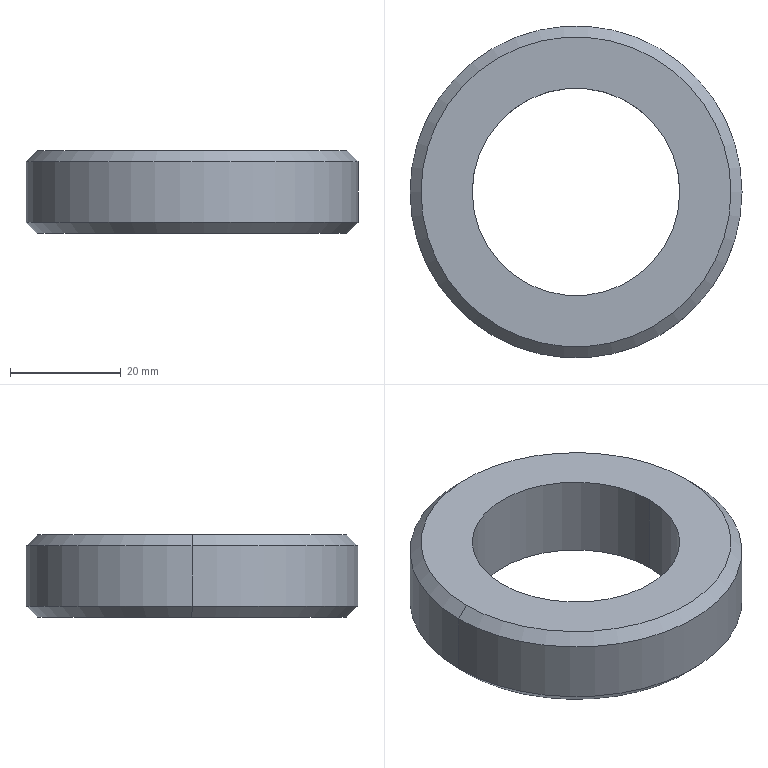Part | SolidWorks | features Chamfer 1, Extrusion 1, HoleWzd 1, ICE 1 | 1 solid | 10 faces | box 60 x 60 x 15 mm | volume 25107 mm3 | cylinder 4 | cone 4 | plane 2 | commonest cylinder face diameters 37.5 x2 60 x2
STEP:
#1=CARTESIAN_POINT('',(-18.75,0.,0.));
#2=VERTEX_POINT('',#1);
#3=CARTESIAN_POINT('',(18.75,0.,0.));
#4=VERTEX_POINT('',#3);
#5=CARTESIAN_POINT('',(0.,0.,0.));
#6=DIRECTION('',(0.,0.,1.));
#7=DIRECTION('',(1.,0.,0.));
#8=AXIS2_PLACEMENT_3D('',#5,#6,#7);
#9=CIRCLE('',#8,18.75);
#10=EDGE_CURVE('',#2,#4,#9,.T.);
#11=ORIENTED_EDGE('',*,*,#10,.F.);
#12=CARTESIAN_POINT('',(-18.75,0.,15.));
#13=VERTEX_POINT('',#12);
#14=CARTESIAN_POINT('',(-18.75,0.,15.));
#15=DIRECTION('',(0.,0.,1.));
#16=VECTOR('',#15,1000.);
#17=LINE('',#14,#16);
#18=EDGE_CURVE('',#2,#13,#17,.T.);
#19=ORIENTED_EDGE('',*,*,#18,.T.);
#20=CARTESIAN_POINT('',(18.75,0.,15.));
#21=VERTEX_POINT('',#20);
#22=CARTESIAN_POINT('',(0.,0.,15.));
#23=DIRECTION('',(0.,0.,1.));
#24=DIRECTION('',(1.,0.,0.));
#25=AXIS2_PLACEMENT_3D('',#22,#23,#24);
#26=CIRCLE('',#25,18.75);
#27=EDGE_CURVE('',#13,#21,#26,.T.);
#28=ORIENTED_EDGE('',*,*,#27,.T.);
#29=CARTESIAN_POINT('',(18.75,0.,15.));
#30=DIRECTION('',(0.,0.,1.));
#31=VECTOR('',#30,1000.);
#32=LINE('',#29,#31);
#33=EDGE_CURVE('',#4,#21,#32,.T.);
#34=ORIENTED_EDGE('',*,*,#33,.F.);
#35=EDGE_LOOP('',(#11,#19,#28,#34));
#36=FACE_OUTER_BOUND('',#35,.T.);
#37=CARTESIAN_POINT('',(0.,0.,15.));
#38=DIRECTION('',(0.,0.,1.));
#39=DIRECTION('',(1.,0.,0.));
#40=AXIS2_PLACEMENT_3D('',#37,#38,#39);
#41=CYLINDRICAL_SURFACE('',#40,18.75);
#42=ADVANCED_FACE('',(#36),#41,.F.);
#43=CARTESIAN_POINT('',(28.,0.,15.));
#44=VERTEX_POINT('',#43);
#45=CARTESIAN_POINT('',(-28.,0.,15.));
#46=VERTEX_POINT('',#45);
#47=CARTESIAN_POINT('',(0.,0.,15.));
#48=DIRECTION('',(0.,0.,1.));
#49=DIRECTION('',(1.,0.,0.));
#50=AXIS2_PLACEMENT_3D('',#47,#48,#49);
#51=CIRCLE('',#50,28.);
#52=EDGE_CURVE('',#44,#46,#51,.T.);
#53=ORIENTED_EDGE('',*,*,#52,.F.);
#54=CARTESIAN_POINT('',(30.,0.,13.));
#55=VERTEX_POINT('',#54);
#56=CARTESIAN_POINT('',(28.,0.,15.));
#57=DIRECTION('',(0.7071,0.,-0.7071));
#58=VECTOR('',#57,1000.);
#59=LINE('',#56,#58);
#60=EDGE_CURVE('',#44,#55,#59,.T.);
#61=ORIENTED_EDGE('',*,*,#60,.T.);
#62=CARTESIAN_POINT('',(-30.,0.,13.));
#63=VERTEX_POINT('',#62);
#64=CARTESIAN_POINT('',(0.,0.,13.));
#65=DIRECTION('',(0.,0.,-1.));
#66=DIRECTION('',(1.,0.,0.));
#67=AXIS2_PLACEMENT_3D('',#64,#65,#66);
#68=CIRCLE('',#67,30.);
#69=EDGE_CURVE('',#63,#55,#68,.T.);
#70=ORIENTED_EDGE('',*,*,#69,.F.);
#71=CARTESIAN_POINT('',(-28.,0.,15.));
#72=DIRECTION('',(-0.7071,0.,-0.7071));
#73=VECTOR('',#72,1000.);
#74=LINE('',#71,#73);
#75=EDGE_CURVE('',#46,#63,#74,.T.);
#76=ORIENTED_EDGE('',*,*,#75,.F.);
#77=EDGE_LOOP('',(#53,#61,#70,#76));
#78=FACE_OUTER_BOUND('',#77,.T.);
#79=CARTESIAN_POINT('',(0.,0.,15.));
#80=DIRECTION('',(0.,0.,-1.));
#81=DIRECTION('',(-1.,0.,0.));
#82=AXIS2_PLACEMENT_3D('',#79,#80,#81);
#83=CONICAL_SURFACE('',#82,28.,0.7854);
#84=ADVANCED_FACE('',(#78),#83,.T.);
#85=CARTESIAN_POINT('',(-28.,0.,0.));
#86=VERTEX_POINT('',#85);
#87=CARTESIAN_POINT('',(28.,0.,0.));
#88=VERTEX_POINT('',#87);
#89=CARTESIAN_POINT('',(0.,0.,0.));
#90=DIRECTION('',(0.,0.,-1.));
#91=DIRECTION('',(1.,0.,0.));
#92=AXIS2_PLACEMENT_3D('',#89,#90,#91);
#93=CIRCLE('',#92,28.);
#94=EDGE_CURVE('',#86,#88,#93,.T.);
#95=ORIENTED_EDGE('',*,*,#94,.F.);
#96=CARTESIAN_POINT('',(-30.,0.,2.));
#97=VERTEX_POINT('',#96);
#98=CARTESIAN_POINT('',(-30.,0.,2.));
#99=DIRECTION('',(-0.7071,0.,0.7071));
#100=VECTOR('',#99,1000.);
#101=LINE('',#98,#100);
#102=EDGE_CURVE('',#86,#97,#101,.T.);
#103=ORIENTED_EDGE('',*,*,#102,.T.);
#104=CARTESIAN_POINT('',(30.,0.,2.));
#105=VERTEX_POINT('',#104);
#106=CARTESIAN_POINT('',(0.,0.,2.));
#107=DIRECTION('',(0.,0.,1.));
#108=DIRECTION('',(1.,0.,0.));
#109=AXIS2_PLACEMENT_3D('',#106,#107,#108);
#110=CIRCLE('',#109,30.);
#111=EDGE_CURVE('',#105,#97,#110,.T.);
#112=ORIENTED_EDGE('',*,*,#111,.F.);
#113=CARTESIAN_POINT('',(30.,0.,2.));
#114=DIRECTION('',(0.7071,0.,0.7071));
#115=VECTOR('',#114,1000.);
#116=LINE('',#113,#115);
#117=EDGE_CURVE('',#88,#105,#116,.T.);
#118=ORIENTED_EDGE('',*,*,#117,.F.);
#119=EDGE_LOOP('',(#95,#103,#112,#118));
#120=FACE_OUTER_BOUND('',#119,.T.);
#121=CARTESIAN_POINT('',(0.,0.,2.));
#122=DIRECTION('',(0.,0.,1.));
#123=DIRECTION('',(1.,0.,0.));
#124=AXIS2_PLACEMENT_3D('',#121,#122,#123);
#125=CONICAL_SURFACE('',#124,30.,0.7854);
#126=ADVANCED_FACE('',(#120),#125,.T.);
#127=ORIENTED_EDGE('',*,*,#69,.T.);
#128=CARTESIAN_POINT('',(30.,0.,15.));
#129=DIRECTION('',(0.,0.,-1.));
#130=VECTOR('',#129,1000.);
#131=LINE('',#128,#130);
#132=EDGE_CURVE('',#55,#105,#131,.T.);
#133=ORIENTED_EDGE('',*,*,#132,.T.);
#134=ORIENTED_EDGE('',*,*,#111,.T.);
#135=CARTESIAN_POINT('',(-30.,0.,15.));
#136=DIRECTION('',(0.,0.,-1.));
#137=VECTOR('',#136,1000.);
#138=LINE('',#135,#137);
#139=EDGE_CURVE('',#63,#97,#138,.T.);
#140=ORIENTED_EDGE('',*,*,#139,.F.);
#141=EDGE_LOOP('',(#127,#133,#134,#140));
#142=FACE_OUTER_BOUND('',#141,.T.);
#143=CARTESIAN_POINT('',(0.,0.,15.));
#144=DIRECTION('',(0.,0.,-1.));
#145=DIRECTION('',(-1.,0.,0.));
#146=AXIS2_PLACEMENT_3D('',#143,#144,#145);
#147=CYLINDRICAL_SURFACE('',#146,30.);
#148=ADVANCED_FACE('',(#142),#147,.T.);
#149=ORIENTED_EDGE('',*,*,#132,.F.);
#150=CARTESIAN_POINT('',(0.,0.,13.));
#151=DIRECTION('',(0.,0.,-1.));
#152=DIRECTION('',(1.,0.,0.));
#153=AXIS2_PLACEMENT_3D('',#150,#151,#152);
#154=CIRCLE('',#153,30.);
#155=EDGE_CURVE('',#55,#63,#154,.T.);
#156=ORIENTED_EDGE('',*,*,#155,.T.);
#157=ORIENTED_EDGE('',*,*,#139,.T.);
#158=CARTESIAN_POINT('',(0.,0.,2.));
#159=DIRECTION('',(0.,0.,1.));
#160=DIRECTION('',(1.,0.,0.));
#161=AXIS2_PLACEMENT_3D('',#158,#159,#160);
#162=CIRCLE('',#161,30.);
#163=EDGE_CURVE('',#97,#105,#162,.T.);
#164=ORIENTED_EDGE('',*,*,#163,.T.);
#165=EDGE_LOOP('',(#149,#156,#157,#164));
#166=FACE_OUTER_BOUND('',#165,.T.);
#167=CARTESIAN_POINT('',(0.,0.,15.));
#168=DIRECTION('',(0.,0.,-1.));
#169=DIRECTION('',(-1.,0.,0.));
#170=AXIS2_PLACEMENT_3D('',#167,#168,#169);
#171=CYLINDRICAL_SURFACE('',#170,30.);
#172=ADVANCED_FACE('',(#166),#171,.T.);
#173=CARTESIAN_POINT('',(0.,0.,15.));
#174=DIRECTION('',(0.,0.,1.));
#175=DIRECTION('',(1.,0.,0.));
#176=AXIS2_PLACEMENT_3D('',#173,#174,#175);
#177=CIRCLE('',#176,18.75);
#178=EDGE_CURVE('',#21,#13,#177,.T.);
#179=ORIENTED_EDGE('',*,*,#178,.F.);
#180=ORIENTED_EDGE('',*,*,#27,.F.);
#181=EDGE_LOOP('',(#179,#180));
#182=FACE_BOUND('',#181,.T.);
#183=CARTESIAN_POINT('',(0.,0.,15.));
#184=DIRECTION('',(0.,0.,1.));
#185=DIRECTION('',(1.,0.,0.));
#186=AXIS2_PLACEMENT_3D('',#183,#184,#185);
#187=CIRCLE('',#186,28.);
#188=EDGE_CURVE('',#46,#44,#187,.T.);
#189=ORIENTED_EDGE('',*,*,#188,.T.);
#190=ORIENTED_EDGE('',*,*,#52,.T.);
#191=EDGE_LOOP('',(#189,#190));
#192=FACE_OUTER_BOUND('',#191,.T.);
#193=CARTESIAN_POINT('',(0.,0.,15.));
#194=DIRECTION('',(0.,0.,1.));
#195=DIRECTION('',(1.,0.,0.));
#196=AXIS2_PLACEMENT_3D('',#193,#194,#195);
#197=PLANE('',#196);
#198=ADVANCED_FACE('',(#182,#192),#197,.T.);
#199=CARTESIAN_POINT('',(0.,0.,0.));
#200=DIRECTION('',(0.,0.,1.));
#201=DIRECTION('',(1.,0.,0.));
#202=AXIS2_PLACEMENT_3D('',#199,#200,#201);
#203=CIRCLE('',#202,18.75);
#204=EDGE_CURVE('',#4,#2,#203,.T.);
#205=ORIENTED_EDGE('',*,*,#204,.T.);
#206=ORIENTED_EDGE('',*,*,#10,.T.);
#207=EDGE_LOOP('',(#205,#206));
#208=FACE_BOUND('',#207,.T.);
#209=CARTESIAN_POINT('',(0.,0.,0.));
#210=DIRECTION('',(0.,0.,-1.));
#211=DIRECTION('',(1.,0.,0.));
#212=AXIS2_PLACEMENT_3D('',#209,#210,#211);
#213=CIRCLE('',#212,28.);
#214=EDGE_CURVE('',#88,#86,#213,.T.);
#215=ORIENTED_EDGE('',*,*,#214,.T.);
#216=ORIENTED_EDGE('',*,*,#94,.T.);
#217=EDGE_LOOP('',(#215,#216));
#218=FACE_OUTER_BOUND('',#217,.T.);
#219=CARTESIAN_POINT('',(0.,0.,0.));
#220=DIRECTION('',(0.,0.,1.));
#221=DIRECTION('',(1.,0.,0.));
#222=AXIS2_PLACEMENT_3D('',#219,#220,#221);
#223=PLANE('',#222);
#224=ADVANCED_FACE('',(#208,#218),#223,.F.);
#225=ORIENTED_EDGE('',*,*,#102,.F.);
#226=ORIENTED_EDGE('',*,*,#214,.F.);
#227=ORIENTED_EDGE('',*,*,#117,.T.);
#228=ORIENTED_EDGE('',*,*,#163,.F.);
#229=EDGE_LOOP('',(#225,#226,#227,#228));
#230=FACE_OUTER_BOUND('',#229,.T.);
#231=CARTESIAN_POINT('',(0.,0.,2.));
#232=DIRECTION('',(0.,0.,1.));
#233=DIRECTION('',(1.,0.,0.));
#234=AXIS2_PLACEMENT_3D('',#231,#232,#233);
#235=CONICAL_SURFACE('',#234,30.,0.7854);
#236=ADVANCED_FACE('',(#230),#235,.T.);
#237=ORIENTED_EDGE('',*,*,#60,.F.);
#238=ORIENTED_EDGE('',*,*,#188,.F.);
#239=ORIENTED_EDGE('',*,*,#75,.T.);
#240=ORIENTED_EDGE('',*,*,#155,.F.);
#241=EDGE_LOOP('',(#237,#238,#239,#240));
#242=FACE_OUTER_BOUND('',#241,.T.);
#243=CARTESIAN_POINT('',(0.,0.,15.));
#244=DIRECTION('',(0.,0.,-1.));
#245=DIRECTION('',(-1.,0.,0.));
#246=AXIS2_PLACEMENT_3D('',#243,#244,#245);
#247=CONICAL_SURFACE('',#246,28.,0.7854);
#248=ADVANCED_FACE('',(#242),#247,.T.);
#249=ORIENTED_EDGE('',*,*,#18,.F.);
#250=ORIENTED_EDGE('',*,*,#204,.F.);
#251=ORIENTED_EDGE('',*,*,#33,.T.);
#252=ORIENTED_EDGE('',*,*,#178,.T.);
#253=EDGE_LOOP('',(#249,#250,#251,#252));
#254=FACE_OUTER_BOUND('',#253,.T.);
#255=CARTESIAN_POINT('',(0.,0.,15.));
#256=DIRECTION('',(0.,0.,1.));
#257=DIRECTION('',(1.,0.,0.));
#258=AXIS2_PLACEMENT_3D('',#255,#256,#257);
#259=CYLINDRICAL_SURFACE('',#258,18.75);
#260=ADVANCED_FACE('',(#254),#259,.F.);
#261=CLOSED_SHELL('',(#42,#84,#126,#148,#172,#198,#224,#236,#248,#260));
#262=MANIFOLD_SOLID_BREP('',#261);
#263=CARTESIAN_POINT('',(0.,0.,0.));
#264=DIRECTION('',(0.,0.,1.));
#265=DIRECTION('',(1.,0.,0.));
#266=AXIS2_PLACEMENT_3D('',#263,#264,#265);
#267=(LENGTH_UNIT()NAMED_UNIT(*)SI_UNIT(.MILLI.,.METRE.));
#268=UNCERTAINTY_MEASURE_WITH_UNIT(LENGTH_MEASURE(0.00001),#267,'','');
#269=(NAMED_UNIT(*)PLANE_ANGLE_UNIT()SI_UNIT($,.RADIAN.));
#270=(NAMED_UNIT(*)SI_UNIT($,.STERADIAN.)SOLID_ANGLE_UNIT());
#271=(GEOMETRIC_REPRESENTATION_CONTEXT(3)GLOBAL_UNCERTAINTY_ASSIGNED_CONTEXT((#268))GLOBAL_UNIT_ASSIGNED_CONTEXT((#267,#269,#270))REPRESENTATION_CONTEXT('',''));
#272=ADVANCED_BREP_SHAPE_REPRESENTATION('',(#262,#266),#271);